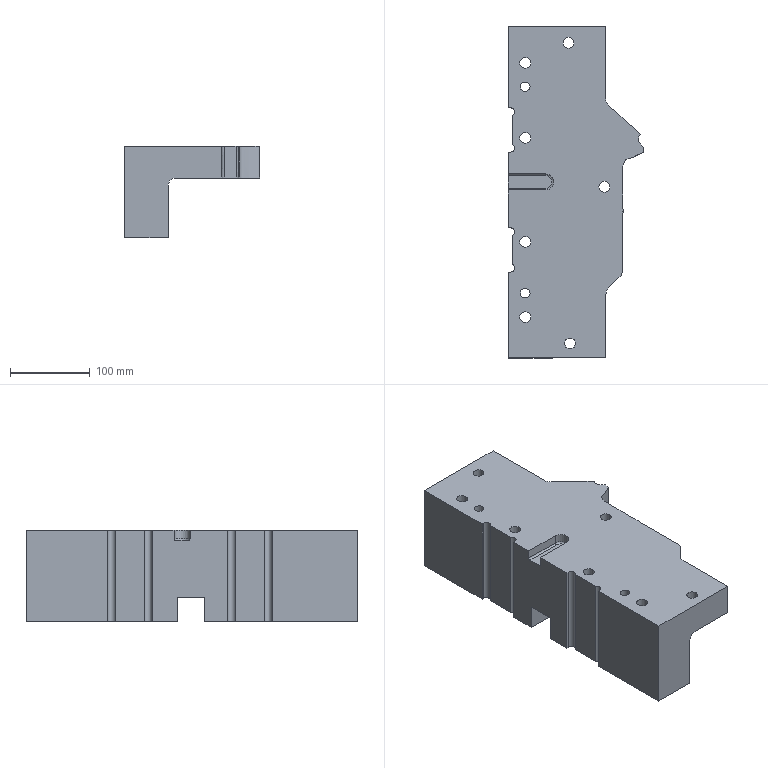Part | NX | features solid 2 | 1 solid | 108 faces | box 169.002 x 415 x 115 mm | volume 3593419 mm3 | cylinder 41 | plane 40 | cone 18 | spline 8 | torus 1 | commonest cylinder face diameters 13.507 x7 20.008 x7 10 x4 10.3 x4 16 x4 4 x2